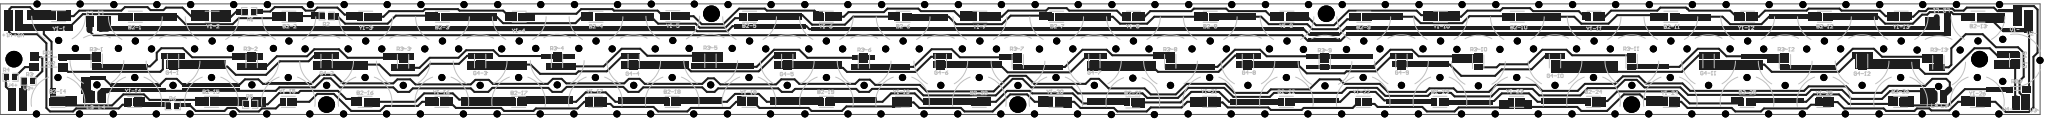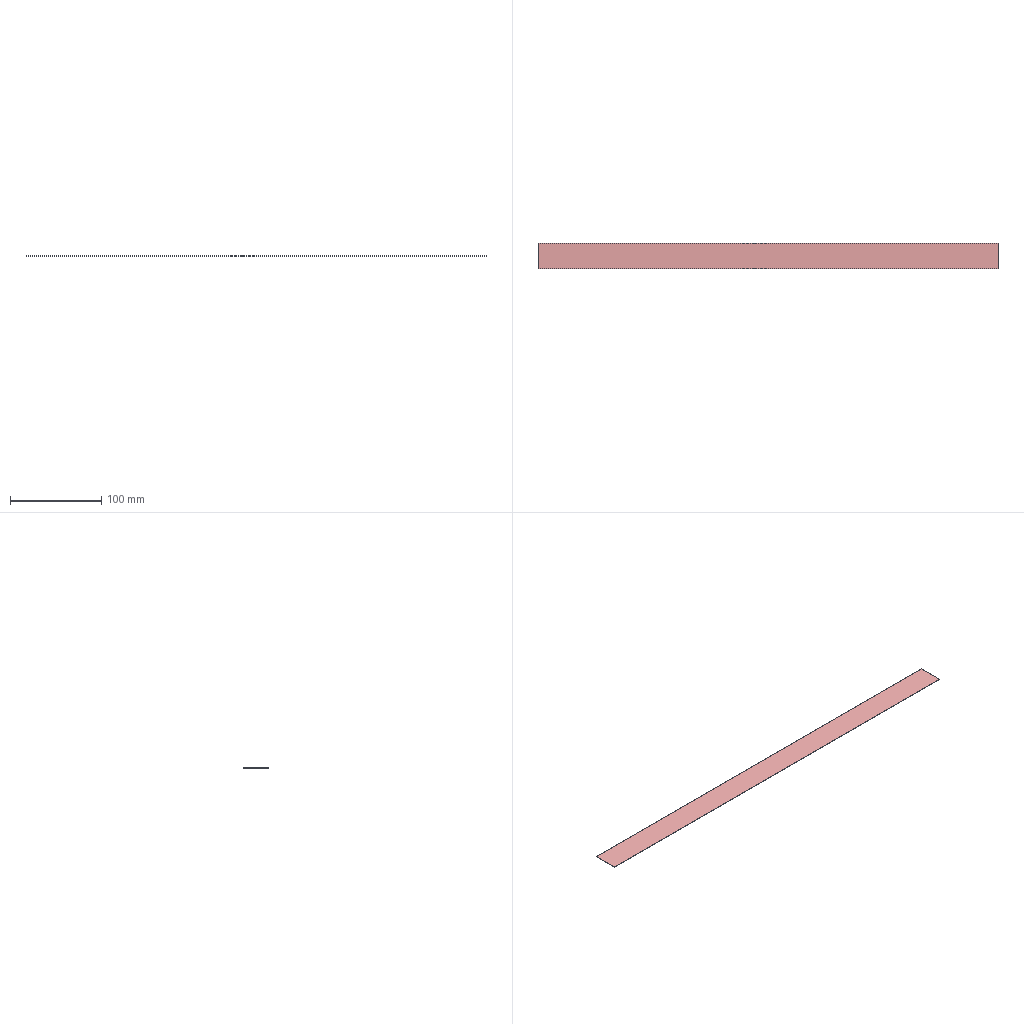Circuit board layout | Altium Designer | box 504.8 x 28 x 0.4 mm
Layer stack:
# Altium Designer layer stack of 10 (unit mm; dielectric type: 0 none, 1 core, 2 prepreg, 3 surface material)
index,name,kind,layer,copper_thickness_mm,dielectric_type,dielectric_thickness_mm,dielectric_material,dielectric_constant
0,Top Paste,other,,,,,,
1,Top Overlay,other,,,,,,
2,Top Solder,dielectric,,,3,0.0102,Solder Resist,3.5
3,Top Layer,copper,Top Layer,0.0356,,,,
4,Dielectric 1,dielectric,,,0,0.32,FR-4,4.8
5,Bottom Layer,copper,Bottom Layer,0.0356,,,,
6,Bottom Solder,dielectric,,,3,0.0102,Solder Resist,3.5
7,Bottom Overlay,other,,,,,,
8,Bottom Paste,other,,,,,,
# drill layer pairs: low layer,high layer
drill_pair,Top Layer,Bottom Layer
Part placement:
Designator,Comment,Layer,Footprint,Center-X(mm),Center-Y(mm),Rotation
Y1-1,2835A03-585Y05-2P-F10,TopLayer,2835LED带透镜1,14.2,24.892,0
R3-2,2835A03-630R05-2P-F10,TopLayer,2835LED带透镜3,62.23,13.328,0
R3-13,2835A03-630R05-2P-F10,TopLayer,2835LED带透镜3,479.65,12.925,0
R3-12,2835A03-630R05-2P-F10,TopLayer,2835LED带透镜3,441.677,13.179,0
R3-11,2835A03-630R05-2P-F10,TopLayer,2835LED带透镜3,403.733,13.201,0
R3-10,2835A03-630R05-2P-F10,TopLayer,2835LED带透镜3,365.76,13.088,0
R3-9,2835A03-630R05-2P-F10,TopLayer,2835LED带透镜3,327.787,13.074,0
R3-8,2835A03-630R05-2P-F10,TopLayer,2835LED带透镜3,289.56,13.201,0
R3-7,2835A03-630R05-2P-F10,TopLayer,2835LED带透镜3,251.812,13.179,0
R3-6,2835A03-630R05-2P-F10,TopLayer,2835LED带透镜3,213.741,13.201,0
R3-5,2835A03-630R05-2P-F10,TopLayer,2835LED带透镜3,175.768,13.328,0
R3-4,2835A03-630R05-2P-F10,TopLayer,2835LED带透镜3,137.795,13.328,0
R3-3,2835A03-630R05-2P-F10,TopLayer,2835LED带透镜3,99.695,13.201,0
R3-1,2835A03-630R05-2P-F10,TopLayer,2835LED带透镜3,23.876,13.328,0
G4-6,2835A03-525G05-2P-F10,TopLayer,2835LED带透镜3,232.775,13.775,0
R02,jumper,TopLayer,贴片跳线QM8.2-D01,12.049,11.992,0
R01,jumper,TopLayer,贴片跳线QM8.2-D01,11.921,14.532,0
R03,jumper,TopLayer,贴片跳线,499.205,6.096,0
R6,20O,TopLayer,R0805,42.697,2.184,0
R5,20O,TopLayer,R0805,61.874,2.565,0
R2,20O,TopLayer,R0805,80.797,24.917,0
R1,20O,TopLayer,R0805,61.62,26.06,0
Y1-26,2835A03-585Y05-2P-F10,TopLayer,2835LED带透镜2,489.048,3.206,0
Y1-25,2835A03-585Y05-2P-F10,TopLayer,2835LED带透镜2,451.048,3.206,0
Y1-24,2835A03-585Y05-2P-F10,TopLayer,2835LED带透镜2,413.048,3.206,0
Y1-23,2835A03-585Y05-2P-F10,TopLayer,2835LED带透镜2,375.048,3.206,0
Y1-22,2835A03-585Y05-2P-F10,TopLayer,2835LED带透镜2,337.048,3.206,0
Y1-21,2835A03-585Y05-2P-F10,TopLayer,2835LED带透镜2,299.048,3.206,0
Y1-20,2835A03-585Y05-2P-F10,TopLayer,2835LED带透镜2,261.033,3.206,0
Y1-19,2835A03-585Y05-2P-F10,TopLayer,2835LED带透镜2,223.048,3.206,0
Y1-18,2835A03-585Y05-2P-F10,TopLayer,2835LED带透镜2,185.048,3.206,0
Y1-17,2835A03-585Y05-2P-F10,TopLayer,2835LED带透镜2,147.048,3.206,0
Y1-16,2835A03-585Y05-2P-F10,TopLayer,2835LED带透镜2,109.048,3.206,0
Y1-15,2835A03-585Y05-2P-F10,TopLayer,2835LED带透镜2,71.048,3.206,0
Y1-14,2835A03-585Y05-2P-F10,TopLayer,2835LED带透镜2,33.048,3.206,0
Y1-13,2835A03-585Y05-2P-F10,TopLayer,2835LED带透镜,470.2,24.747,0
Y1-12,2835A03-585Y05-2P-F10,TopLayer,2835LED带透镜,432.2,24.747,0
Y1-11,2835A03-585Y05-2P-F10,TopLayer,2835LED带透镜,394.2,24.747,0
Y1-10,2835A03-585Y05-2P-F10,TopLayer,2835LED带透镜,356.2,24.747,0
Y1-9,2835A03-585Y05-2P-F10,TopLayer,2835LED带透镜,318.2,24.747,0
Y1-8,2835A03-585Y05-2P-F10,TopLayer,2835LED带透镜,280.2,24.747,0
Y1-7,2835A03-585Y05-2P-F10,TopLayer,2835LED带透镜,242.2,24.747,0
Y1-6,2835A03-585Y05-2P-F10,TopLayer,2835LED带透镜,204.2,24.747,0
Y1-5,2835A03-585Y05-2P-F10,TopLayer,2835LED带透镜,166.2,24.874,0
Y1-4,2835A03-585Y05-2P-F10,TopLayer,2835LED带透镜,128.2,24.747,0
Y1-3,2835A03-585Y05-2P-F10,TopLayer,2835LED带透镜,90.2,24.747,0
Y1-2,2835A03-585Y05-2P-F10,TopLayer,2835LED带透镜,52.2,24.747,0
R4,10O,TopLayer,R0805,2.565,9.423,0
R3,10O,TopLayer,R0805,7.01,8.407,0
G4-13,2835A03-525G05-2P-F10,TopLayer,2835LED带透镜2,498.65,13.952,270
G4-12,2835A03-525G05-2P-F10,TopLayer,2835LED带透镜3,460.775,13.775,0
G4-11,2835A03-525G05-2P-F10,TopLayer,2835LED带透镜3,422.775,13.775,0
G4-10,2835A03-525G05-2P-F10,TopLayer,2835LED带透镜3,384.775,13.775,0
G4-9,2835A03-525G05-2P-F10,TopLayer,2835LED带透镜3,346.775,13.775,0
G4-8,2835A03-525G05-2P-F10,TopLayer,2835LED带透镜3,308.775,13.775,0
G4-7,2835A03-525G05-2P-F10,TopLayer,2835LED带透镜3,270.775,13.775,0
G4-5,2835A03-525G05-2P-F10,TopLayer,2835LED带透镜3,194.775,13.775,0
G4-4,2835A03-525G05-2P-F10,TopLayer,2835LED带透镜3,156.775,13.775,0
G4-3,2835A03-525G05-2P-F10,TopLayer,2835LED带透镜3,118.775,13.775,0
G4-2,2835A03-525G05-2P-F10,TopLayer,2835LED带透镜3,80.775,13.775,0
G4-1,2835A03-525G05-2P-F10,TopLayer,2835LED带透镜3,42.775,13.775,0
B2-13,2835A03-480B05-1S-F8,TopLayer,2835LED带透镜,489.2,24.765,0
B2-12,2835A03-480B05-1S-F8,TopLayer,2835LED带透镜,451.2,24.747,0
B2-11,2835A03-480B05-1S-F8,TopLayer,2835LED带透镜,413.2,24.747,0
B2-10,2835A03-480B05-1S-F8,TopLayer,2835LED带透镜,375.2,24.747,0
B2-9,2835A03-480B05-1S-F8,TopLayer,2835LED带透镜,337.2,24.747,0
B2-8,2835A03-480B05-1S-F8,TopLayer,2835LED带透镜,299.2,24.747,0
B2-7,2835A03-480B05-1S-F8,TopLayer,2835LED带透镜,261.2,24.747,0
B2-6,2835A03-480B05-1S-F8,TopLayer,2835LED带透镜,223.2,24.747,0
B2-5,2835A03-480B05-1S-F8,TopLayer,2835LED带透镜,185.2,24.747,0
B2-4,2835A03-480B05-1S-F8,TopLayer,2835LED带透镜,147.2,24.747,0
B2-3,2835A03-480B05-1S-F8,TopLayer,2835LED带透镜,109.2,24.747,0
B2-2,2835A03-480B05-1S-F8,TopLayer,2835LED带透镜,71.2,24.747,0
B2-1,2835A03-480B05-1S-F8,TopLayer,2835LED带透镜,33.2,24.747,0
B2-26,2835A03-480B05-1S-F8,TopLayer,2835LED带透镜2,470.048,3.206,0
B2-25,2835A03-480B05-1S-F8,TopLayer,2835LED带透镜2,432.048,3.206,0
B2-24,2835A03-480B05-1S-F8,TopLayer,2835LED带透镜2,394.048,3.206,0
B2-23,2835A03-480B05-1S-F8,TopLayer,2835LED带透镜2,356.048,3.206,0
B2-22,2835A03-480B05-1S-F8,TopLayer,2835LED带透镜2,318.048,3.206,0
B2-21,2835A03-480B05-1S-F8,TopLayer,2835LED带透镜2,280.048,3.048,0
B2-20,2835A03-480B05-1S-F8,TopLayer,2835LED带透镜2,242.048,3.206,0
B2-19,2835A03-480B05-1S-F8,TopLayer,2835LED带透镜2,204.223,3.206,0
B2-18,2835A03-480B05-1S-F8,TopLayer,2835LED带透镜2,166.048,3.206,0
B2-17,2835A03-480B05-1S-F8,TopLayer,2835LED带透镜2,128.048,3.206,0
B2-16,2835A03-480B05-1S-F8,TopLayer,2835LED带透镜2,90.048,3.206,0
B2-15,2835A03-480B05-1S-F8,TopLayer,2835LED带透镜2,52.048,3.206,0
B2-14,2835A03-480B05-1S-F8,TopLayer,2835LED带透镜2,14.048,3.206,0
Pad and via stacks:
# Altium Designer via and pad stacks of 10 (unit mm). Each distinct definition once, with the count of objects using it.
# via: kind,start_layer,end_layer,hole_mm,diameter_mm,mode(0 simple;1 top-mid-bottom;2 full stack),diameter_per_layer,count,example_net
# pad: kind,layer,hole_mm,hole_type(0 round;1 square;2 slot),plating,top_size,top_shape(1 round;2 rect;3 octagon;9 rounded rect),mid_size,bottom_size,mode,footprint,size_per_layer,count,example
pad,Top Layer,0,0,plated,1.5x4,1,1.5x4,1.5x4,0,,,1,0
pad,Top Layer,0,0,plated,1.5x3.3,1,1.5x3.3,1.5x3.3,0,,,4,0
pad,Top Layer,0,0,plated,1.2x2.6,1,1.2x2.6,1.2x2.6,0,,,2,0
pad,Top Layer,0,0,plated,1.5x3,1,1.5x3,1.5x3,0,,,2,0
pad,Top Layer,0,0,plated,1.5x3.8,1,1.5x3.8,1.5x3.8,0,,,1,0
pad,Top Layer,0,0,plated,1.5x3.75,1,1.5x3.75,1.5x3.75,0,,,2,0
pad,Top Layer,0,0,plated,1.3x3,1,1.3x3,1.3x3,0,,,2,0
pad,Top Layer,0,0,plated,1.8x1.7,2,1.8x1.7,1.8x1.7,0,\u00CC\u00F9\u00C6\u00AC\u00CC\u00F8\u00CF\u00DFQM8.2-D01,,4,R01.2
pad,Top Layer,0,0,plated,1x1.27,2,1x1.27,1x1.27,0,R0805,,12,R3.1
pad,Top Layer,0,0,plated,1.5x3.6,1,1.5x3.6,1.5x3.6,0,,,2,0
pad,Top Layer,0,0,plated,1.5x1.2,2,1.5x1.2,1.5x1.2,0,\u00CC\u00F9\u00C6\u00AC\u00CC\u00F8\u00CF\u00DF,,2,R03.2
pad,Top Layer,0,0,plated,2x1.3,2,2x1.3,2x1.3,0,2835LED\u00B4\u00F8\u00CD\u00B8\u00BE\u00B53,,25,R3-2.1
pad,Top Layer,0,0,plated,2x2.3,2,2x2.3,2x2.3,0,2835LED\u00B4\u00F8\u00CD\u00B8\u00BE\u00B53,,25,R3-2.2
pad,Top Layer,0,0,plated,2x1.3,2,2x1.3,2x1.3,0,2835LED\u00B4\u00F8\u00CD\u00B8\u00BE\u00B52,,27,G4-13.1
pad,Top Layer,0,0,plated,2x2.3,2,2x2.3,2x2.3,0,2835LED\u00B4\u00F8\u00CD\u00B8\u00BE\u00B52,,27,G4-13.2
pad,Top Layer,0,0,plated,2x2.3,2,2x2.3,2x2.3,0,2835LED\u00B4\u00F8\u00CD\u00B8\u00BE\u00B5,,26,B2-1.2
pad,Top Layer,0,0,plated,2x1.3,2,2x1.3,2x1.3,0,2835LED\u00B4\u00F8\u00CD\u00B8\u00BE\u00B5,,26,B2-1.1
pad,Top Layer,0,0,plated,1.5x5,1,1.5x5,1.5x5,0,,,6,0
via,Top Layer,Bottom Layer,3,4.2,0,,7,
via,Top Layer,Bottom Layer,1.8,1.8,0,,234,
Design rules, without the lines most boards share:
# Altium Designer design rules of 10 (exported by Altium Designer, unit mm)
# columns: name | kind | enabled | priority | scope1 | scope2 | descriptor | typed fields (field=value)
Sheet1 | 22 | enabled | 1 | InComponentClass('Sheet1') | All | Room Sheet1 (Bounding Region = (0mm, 0mm, 50.8mm, 25.4mm) (InComponentClass('Sheet1')) |
NetAntennae | 56 | enabled | 1 | All | All | Net Antennae (Tolerance=0mm) (All) |
SilkToSilkClearance | 55 | enabled | 1 | All | All | Silk to Silk (Clearance=0mm) (All),(All) |
SilkToSolderMaskClearance | 54 | enabled | 1 | IsPad | All | Silk To Solder Mask (Clearance=0mm) (IsPad),(All) |
MinimumSolderMaskSliver | 53 | enabled | 1 | All | All | Minimum Solder Mask Sliver (Gap=0mm) (All),(All) |
HoleToHoleClearance | 52 | enabled | 1 | All | All | Hole To Hole Clearance (Gap=0mm) (All),(All) | gap=0
DiffPairsRouting | 51 | enabled | 1 | All | All | Differential Pairs Uncoupled Length using the Gap Constraints (Min=0.254mm) (Max=0.254mm) (Prefered=0.254mm)  and Width Constraints (Min=0.381mm) (Max=0.381mm) (Prefered=0.381mm) (All) |
HoleSize | 42 | enabled | 1 | All | All | Hole Size Constraint (Min=0.025mm) (Max=25.4mm) (All) |
Height | 50 | enabled | 1 | All | All | Height Constraint (Min=0mm) (Max=25.4mm) (Prefered=12.7mm) (All) | min_height=0 max_height=25.4
ComponentClearance | 24 | enabled | 1 | All | All | Component Clearance Constraint ( Horizontal Gap = 0mm, Vertical Gap = 0mm ) (All),(All)  | gap=0
SolderMaskExpansion | 13 | enabled | 1 | All | All | Solder Mask Expansion (Expansion =0.102mm) (All) | expansion=0.1016
PasteMaskExpansion | 14 | enabled | 1 | All | All | Paste Mask Expansion (Expansion =0mm) (All) | expansion=0
RoutingVias | 11 | enabled | 1 | All | All | Routing Via (MinHoleWidth=0.1mm) (MaxHoleWidth=50mm) (PreferredHoleWidth=0.711mm) (MinWidth=0.1mm) (MaxWidth=50mm) (PreferedWidth=1.27mm) (All) | via_min_hole=0.1 via_max_hole=50 via_preferred_diameter=1.27 via_preferred_hole=0.7112
RoutingCorners | 10 | enabled | 1 | All | All | Routing Corners (Style=45-Degree) (Min Setback=2.54mm) (Max Setback=2.54mm) (All) |
Width | 2 | enabled | 1 | All | All | Width Constraint (Min=0.254mm) (Max=2.54mm) (Preferred=0.508mm) (All) |
PolygonConnect | 20 | enabled | 1 | All | All | Polygon Connect Rule(Relief Connect )(Conductor Width=0.254mm) (Relief Angle=90 Angle) (Entries=4) (Air Gap Width=0.254mm) (All),(All) | connect_style(0=relief,1=direct,2=none)=0 relief_conductor_width=0.254 relief_entries=4
PlaneClearance | 12 | enabled | 1 | All | All | Power Plane Clearance (Clearance =0.508mm) (All) | clearance=0.508
PlaneConnect | 6 | enabled | 1 | All | All | Power Plane Connect Rule(Relief Connect )(Expansion=0.508mm) (Conductor Width=0.254mm) (Air Gap=0.254mm) (Entries=4) (All) | relief_conductor_width=0.254 relief_entries=4 relief_expansion=0.508
Clearance | 0 | enabled | 1 | All | All | Clearance Constraint (Gap=0mm) (All),(All) | gap=0
Classes set for this board:
# Altium Designer classes of 10 (member kind: 0 net, 1 component, 2 from-to, 3 pad, 4 layer, 5 differential pair, 6 design channel, 7 polygon, 8 structure, 9 xSignal)
# columns: class name | member kind | superclass | members
Sheet1 | 1 | no | B2-1; B2-2; B2-3; B2-4; B2-5; B2-6; B2-7; B2-8; B2-9; B2-10; B2-11; B2-12; B2-13; G4-1; G4-2; G4-3; G4-4; G4-5; G4-6; G4-7; G4-8; G4-9; G4-10; G4-11; G4-12; G4-13; R3; R3-1; R3-3; R3-4; R3-5; R3-6; R3-7; R3-8; R3-9; R3-10; R3-11; R3-12; R3-13; R4; Y1-1; Y1-2; Y1-3; Y1-4; Y1-5; Y1-6; Y1-7; Y1-8; Y1-9; Y1-10; Y1-11; Y1-12; Y1-13; Y1-14; Y1-15; Y1-16; Y1-17; Y1-18; Y1-19; Y1-20; Y1-21; Y1-22; Y1-23; Y1-24; Y1-25; Y1-26; B2-26; B2-14; B2-15; B2-16; B2-18; B2-22; B2-24; B2-25; B2-17; B2-19; B2-20; B2-21; B2-23; R3-2; R1; R2; R5; R6; R01; R02; R03;